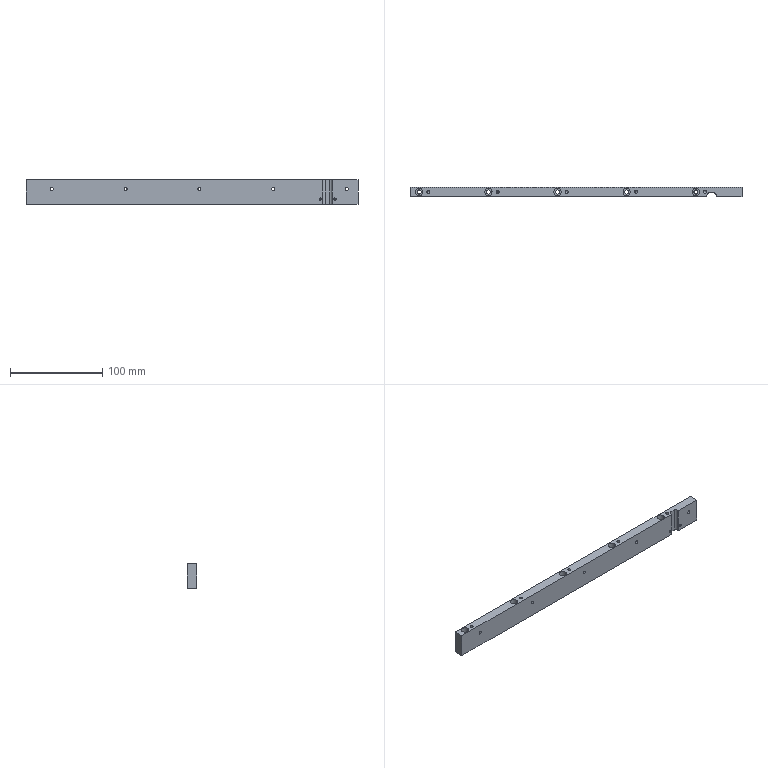Part | NX | features BREP 1 | 1 solid | 75 faces | box 360 x 10 x 26.5 mm | volume 89636 mm3 | cylinder 46 | plane 15 | cone 14 | commonest cylinder face diameters 3.3 x20 4.5 x10 8 x10 2.5 x4 5 x2